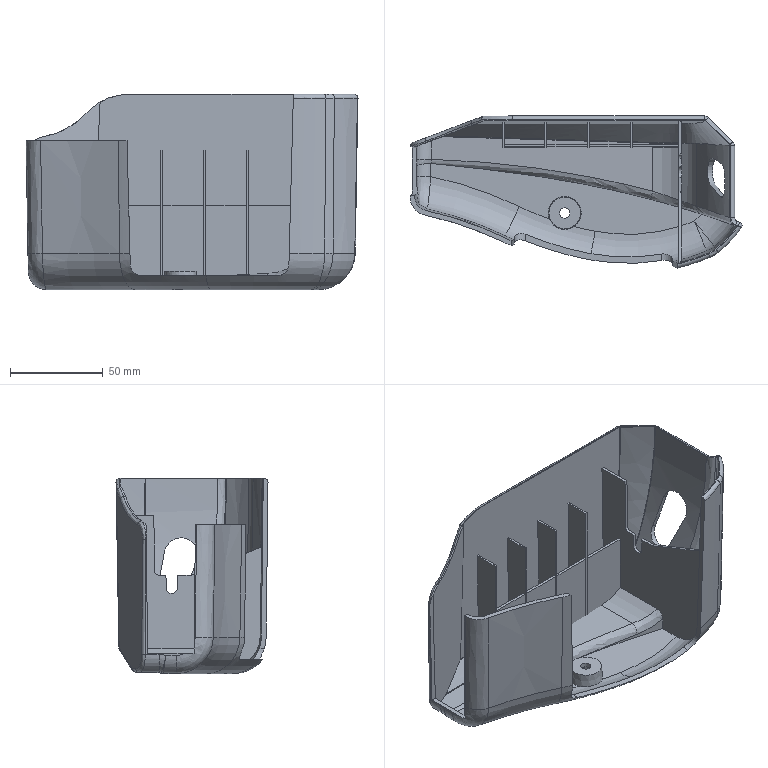Part | STEP file | END CAP R | 1 solid | 190 faces | box 178.531 x 81.742 x 105 mm | volume 112295 mm3 | plane 67 | spline 66 | cylinder 27 | torus 14 | cone 12 | sphere 4 | commonest cylinder face diameters 4 x7 15 x3 55 x3 12 x2 20 x2 1035 x2